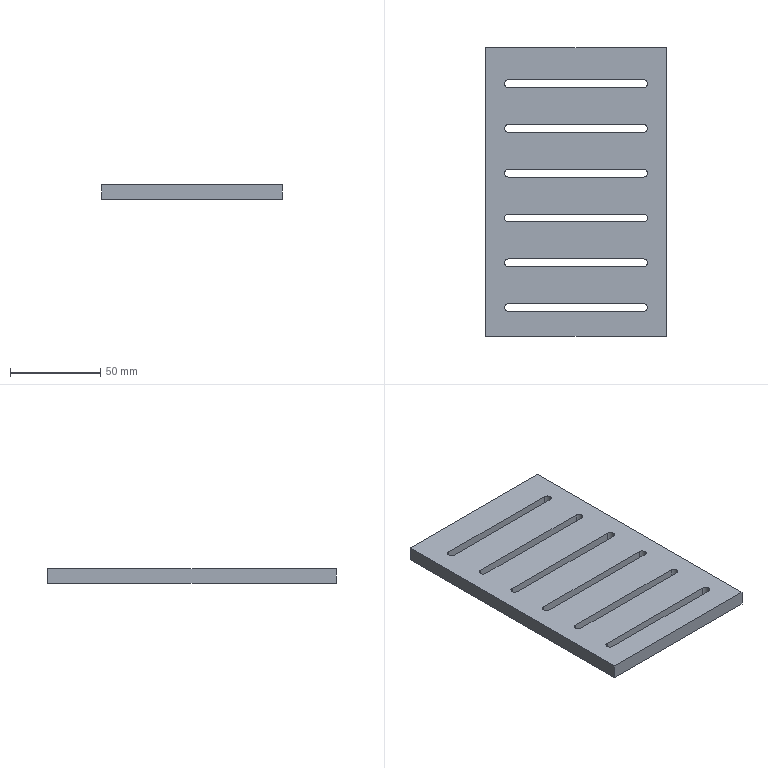Part | STEP file | SynoNew-0304-040 | 1 solid | 38 faces | box 100 x 160 x 8 mm | volume 111423 mm3 | plane 18 | cylinder 16 | cone 4 | commonest cylinder face diameters 4.3 x12 3.242 x4
STEP:
#1=CARTESIAN_POINT('',(-11.379,68.2,4.));
#2=VERTEX_POINT('',#1);
#3=CARTESIAN_POINT('',(-14.621,68.2,4.));
#4=VERTEX_POINT('',#3);
#5=CARTESIAN_POINT('',(-13.,68.2,4.));
#6=DIRECTION('',(0.,1.,0.));
#7=DIRECTION('',(1.,0.,0.));
#8=AXIS2_PLACEMENT_3D('',#5,#6,#7);
#9=CIRCLE('',#8,1.621);
#10=EDGE_CURVE('',#2,#4,#9,.T.);
#11=ORIENTED_EDGE('',*,*,#10,.T.);
#12=CARTESIAN_POINT('',(-13.,67.226,4.));
#13=VERTEX_POINT('',#12);
#14=CARTESIAN_POINT('',(-13.81,67.713,4.));
#15=DIRECTION('',(0.8572,-0.515,0.));
#16=VECTOR('',#15,0.8105);
#17=LINE('',#14,#16);
#18=EDGE_CURVE('',#4,#13,#17,.T.);
#19=ORIENTED_EDGE('',*,*,#18,.T.);
#20=ORIENTED_EDGE('',*,*,#18,.F.);
#21=CARTESIAN_POINT('',(-13.,68.2,4.));
#22=DIRECTION('',(0.,1.,0.));
#23=DIRECTION('',(1.,0.,0.));
#24=AXIS2_PLACEMENT_3D('',#21,#22,#23);
#25=CIRCLE('',#24,1.621);
#26=EDGE_CURVE('',#4,#2,#25,.T.);
#27=ORIENTED_EDGE('',*,*,#26,.T.);
#28=EDGE_LOOP('',(#11,#19,#20,#27));
#29=FACE_OUTER_BOUND('',#28,.T.);
#30=CARTESIAN_POINT('',(-13.,67.713,4.));
#31=DIRECTION('',(0.,1.,0.));
#32=DIRECTION('',(1.,0.,0.));
#33=AXIS2_PLACEMENT_3D('',#30,#31,#32);
#34=CONICAL_SURFACE('',#33,0.8105,1.03);
#35=ADVANCED_FACE('',(#29),#34,.F.);
#36=CARTESIAN_POINT('',(-11.379,80.,4.));
#37=VERTEX_POINT('',#36);
#38=CARTESIAN_POINT('',(-14.621,80.,4.));
#39=VERTEX_POINT('',#38);
#40=CARTESIAN_POINT('',(-13.,80.,4.));
#41=DIRECTION('',(0.,-1.,0.));
#42=DIRECTION('',(1.,0.,0.));
#43=AXIS2_PLACEMENT_3D('',#40,#41,#42);
#44=CIRCLE('',#43,1.621);
#45=EDGE_CURVE('',#37,#39,#44,.T.);
#46=ORIENTED_EDGE('',*,*,#45,.F.);
#47=CARTESIAN_POINT('',(-13.,80.,4.));
#48=DIRECTION('',(0.,-1.,0.));
#49=DIRECTION('',(1.,0.,0.));
#50=AXIS2_PLACEMENT_3D('',#47,#48,#49);
#51=CIRCLE('',#50,1.621);
#52=EDGE_CURVE('',#39,#37,#51,.T.);
#53=ORIENTED_EDGE('',*,*,#52,.F.);
#54=CARTESIAN_POINT('',(-14.621,74.1,4.));
#55=DIRECTION('',(0.,-1.,0.));
#56=VECTOR('',#55,1.621);
#57=LINE('',#54,#56);
#58=EDGE_CURVE('',#39,#4,#57,.T.);
#59=ORIENTED_EDGE('',*,*,#58,.T.);
#60=ORIENTED_EDGE('',*,*,#10,.F.);
#61=ORIENTED_EDGE('',*,*,#26,.F.);
#62=ORIENTED_EDGE('',*,*,#58,.F.);
#63=EDGE_LOOP('',(#46,#53,#59,#60,#61,#62));
#64=FACE_OUTER_BOUND('',#63,.T.);
#65=CARTESIAN_POINT('',(-13.,74.1,4.));
#66=DIRECTION('',(0.,1.,0.));
#67=DIRECTION('',(1.,0.,0.));
#68=AXIS2_PLACEMENT_3D('',#65,#66,#67);
#69=CYLINDRICAL_SURFACE('',#68,1.621);
#70=ADVANCED_FACE('',(#64),#69,.F.);
#71=CARTESIAN_POINT('',(39.621,68.2,4.));
#72=VERTEX_POINT('',#71);
#73=CARTESIAN_POINT('',(36.379,68.2,4.));
#74=VERTEX_POINT('',#73);
#75=CARTESIAN_POINT('',(38.,68.2,4.));
#76=DIRECTION('',(0.,1.,0.));
#77=DIRECTION('',(1.,0.,0.));
#78=AXIS2_PLACEMENT_3D('',#75,#76,#77);
#79=CIRCLE('',#78,1.621);
#80=EDGE_CURVE('',#72,#74,#79,.T.);
#81=ORIENTED_EDGE('',*,*,#80,.T.);
#82=CARTESIAN_POINT('',(38.,67.226,4.));
#83=VERTEX_POINT('',#82);
#84=CARTESIAN_POINT('',(37.19,67.713,4.));
#85=DIRECTION('',(0.8572,-0.515,0.));
#86=VECTOR('',#85,0.8105);
#87=LINE('',#84,#86);
#88=EDGE_CURVE('',#74,#83,#87,.T.);
#89=ORIENTED_EDGE('',*,*,#88,.T.);
#90=ORIENTED_EDGE('',*,*,#88,.F.);
#91=CARTESIAN_POINT('',(38.,68.2,4.));
#92=DIRECTION('',(0.,1.,0.));
#93=DIRECTION('',(1.,0.,0.));
#94=AXIS2_PLACEMENT_3D('',#91,#92,#93);
#95=CIRCLE('',#94,1.621);
#96=EDGE_CURVE('',#74,#72,#95,.T.);
#97=ORIENTED_EDGE('',*,*,#96,.T.);
#98=EDGE_LOOP('',(#81,#89,#90,#97));
#99=FACE_OUTER_BOUND('',#98,.T.);
#100=CARTESIAN_POINT('',(38.,67.713,4.));
#101=DIRECTION('',(0.,1.,0.));
#102=DIRECTION('',(1.,0.,0.));
#103=AXIS2_PLACEMENT_3D('',#100,#101,#102);
#104=CONICAL_SURFACE('',#103,0.8105,1.03);
#105=ADVANCED_FACE('',(#99),#104,.F.);
#106=CARTESIAN_POINT('',(39.621,80.,4.));
#107=VERTEX_POINT('',#106);
#108=CARTESIAN_POINT('',(36.379,80.,4.));
#109=VERTEX_POINT('',#108);
#110=CARTESIAN_POINT('',(38.,80.,4.));
#111=DIRECTION('',(0.,-1.,0.));
#112=DIRECTION('',(1.,0.,0.));
#113=AXIS2_PLACEMENT_3D('',#110,#111,#112);
#114=CIRCLE('',#113,1.621);
#115=EDGE_CURVE('',#107,#109,#114,.T.);
#116=ORIENTED_EDGE('',*,*,#115,.F.);
#117=CARTESIAN_POINT('',(38.,80.,4.));
#118=DIRECTION('',(0.,-1.,0.));
#119=DIRECTION('',(1.,0.,0.));
#120=AXIS2_PLACEMENT_3D('',#117,#118,#119);
#121=CIRCLE('',#120,1.621);
#122=EDGE_CURVE('',#109,#107,#121,.T.);
#123=ORIENTED_EDGE('',*,*,#122,.F.);
#124=CARTESIAN_POINT('',(36.379,74.1,4.));
#125=DIRECTION('',(0.,-1.,0.));
#126=VECTOR('',#125,1.621);
#127=LINE('',#124,#126);
#128=EDGE_CURVE('',#109,#74,#127,.T.);
#129=ORIENTED_EDGE('',*,*,#128,.T.);
#130=ORIENTED_EDGE('',*,*,#80,.F.);
#131=ORIENTED_EDGE('',*,*,#96,.F.);
#132=ORIENTED_EDGE('',*,*,#128,.F.);
#133=EDGE_LOOP('',(#116,#123,#129,#130,#131,#132));
#134=FACE_OUTER_BOUND('',#133,.T.);
#135=CARTESIAN_POINT('',(38.,74.1,4.));
#136=DIRECTION('',(0.,1.,0.));
#137=DIRECTION('',(1.,0.,0.));
#138=AXIS2_PLACEMENT_3D('',#135,#136,#137);
#139=CYLINDRICAL_SURFACE('',#138,1.621);
#140=ADVANCED_FACE('',(#134),#139,.F.);
#141=CARTESIAN_POINT('',(14.621,68.2,4.));
#142=VERTEX_POINT('',#141);
#143=CARTESIAN_POINT('',(11.379,68.2,4.));
#144=VERTEX_POINT('',#143);
#145=CARTESIAN_POINT('',(13.,68.2,4.));
#146=DIRECTION('',(0.,1.,0.));
#147=DIRECTION('',(1.,0.,0.));
#148=AXIS2_PLACEMENT_3D('',#145,#146,#147);
#149=CIRCLE('',#148,1.621);
#150=EDGE_CURVE('',#142,#144,#149,.T.);
#151=ORIENTED_EDGE('',*,*,#150,.T.);
#152=CARTESIAN_POINT('',(13.,67.226,4.));
#153=VERTEX_POINT('',#152);
#154=CARTESIAN_POINT('',(12.19,67.713,4.));
#155=DIRECTION('',(0.8572,-0.515,0.));
#156=VECTOR('',#155,0.8105);
#157=LINE('',#154,#156);
#158=EDGE_CURVE('',#144,#153,#157,.T.);
#159=ORIENTED_EDGE('',*,*,#158,.T.);
#160=ORIENTED_EDGE('',*,*,#158,.F.);
#161=CARTESIAN_POINT('',(13.,68.2,4.));
#162=DIRECTION('',(0.,1.,0.));
#163=DIRECTION('',(1.,0.,0.));
#164=AXIS2_PLACEMENT_3D('',#161,#162,#163);
#165=CIRCLE('',#164,1.621);
#166=EDGE_CURVE('',#144,#142,#165,.T.);
#167=ORIENTED_EDGE('',*,*,#166,.T.);
#168=EDGE_LOOP('',(#151,#159,#160,#167));
#169=FACE_OUTER_BOUND('',#168,.T.);
#170=CARTESIAN_POINT('',(13.,67.713,4.));
#171=DIRECTION('',(0.,1.,0.));
#172=DIRECTION('',(1.,0.,0.));
#173=AXIS2_PLACEMENT_3D('',#170,#171,#172);
#174=CONICAL_SURFACE('',#173,0.8105,1.03);
#175=ADVANCED_FACE('',(#169),#174,.F.);
#176=CARTESIAN_POINT('',(14.621,80.,4.));
#177=VERTEX_POINT('',#176);
#178=CARTESIAN_POINT('',(11.379,80.,4.));
#179=VERTEX_POINT('',#178);
#180=CARTESIAN_POINT('',(13.,80.,4.));
#181=DIRECTION('',(0.,-1.,0.));
#182=DIRECTION('',(1.,0.,0.));
#183=AXIS2_PLACEMENT_3D('',#180,#181,#182);
#184=CIRCLE('',#183,1.621);
#185=EDGE_CURVE('',#177,#179,#184,.T.);
#186=ORIENTED_EDGE('',*,*,#185,.F.);
#187=CARTESIAN_POINT('',(13.,80.,4.));
#188=DIRECTION('',(0.,-1.,0.));
#189=DIRECTION('',(1.,0.,0.));
#190=AXIS2_PLACEMENT_3D('',#187,#188,#189);
#191=CIRCLE('',#190,1.621);
#192=EDGE_CURVE('',#179,#177,#191,.T.);
#193=ORIENTED_EDGE('',*,*,#192,.F.);
#194=CARTESIAN_POINT('',(11.379,74.1,4.));
#195=DIRECTION('',(0.,-1.,0.));
#196=VECTOR('',#195,1.621);
#197=LINE('',#194,#196);
#198=EDGE_CURVE('',#179,#144,#197,.T.);
#199=ORIENTED_EDGE('',*,*,#198,.T.);
#200=ORIENTED_EDGE('',*,*,#150,.F.);
#201=ORIENTED_EDGE('',*,*,#166,.F.);
#202=ORIENTED_EDGE('',*,*,#198,.F.);
#203=EDGE_LOOP('',(#186,#193,#199,#200,#201,#202));
#204=FACE_OUTER_BOUND('',#203,.T.);
#205=CARTESIAN_POINT('',(13.,74.1,4.));
#206=DIRECTION('',(0.,1.,0.));
#207=DIRECTION('',(1.,0.,0.));
#208=AXIS2_PLACEMENT_3D('',#205,#206,#207);
#209=CYLINDRICAL_SURFACE('',#208,1.621);
#210=ADVANCED_FACE('',(#204),#209,.F.);
#211=CARTESIAN_POINT('',(-36.379,68.2,4.));
#212=VERTEX_POINT('',#211);
#213=CARTESIAN_POINT('',(-39.621,68.2,4.));
#214=VERTEX_POINT('',#213);
#215=CARTESIAN_POINT('',(-38.,68.2,4.));
#216=DIRECTION('',(0.,1.,0.));
#217=DIRECTION('',(1.,0.,0.));
#218=AXIS2_PLACEMENT_3D('',#215,#216,#217);
#219=CIRCLE('',#218,1.621);
#220=EDGE_CURVE('',#212,#214,#219,.T.);
#221=ORIENTED_EDGE('',*,*,#220,.T.);
#222=CARTESIAN_POINT('',(-38.,67.226,4.));
#223=VERTEX_POINT('',#222);
#224=CARTESIAN_POINT('',(-38.81,67.713,4.));
#225=DIRECTION('',(0.8572,-0.515,0.));
#226=VECTOR('',#225,0.8105);
#227=LINE('',#224,#226);
#228=EDGE_CURVE('',#214,#223,#227,.T.);
#229=ORIENTED_EDGE('',*,*,#228,.T.);
#230=ORIENTED_EDGE('',*,*,#228,.F.);
#231=CARTESIAN_POINT('',(-38.,68.2,4.));
#232=DIRECTION('',(0.,1.,0.));
#233=DIRECTION('',(1.,0.,0.));
#234=AXIS2_PLACEMENT_3D('',#231,#232,#233);
#235=CIRCLE('',#234,1.621);
#236=EDGE_CURVE('',#214,#212,#235,.T.);
#237=ORIENTED_EDGE('',*,*,#236,.T.);
#238=EDGE_LOOP('',(#221,#229,#230,#237));
#239=FACE_OUTER_BOUND('',#238,.T.);
#240=CARTESIAN_POINT('',(-38.,67.713,4.));
#241=DIRECTION('',(0.,1.,0.));
#242=DIRECTION('',(1.,0.,0.));
#243=AXIS2_PLACEMENT_3D('',#240,#241,#242);
#244=CONICAL_SURFACE('',#243,0.8105,1.03);
#245=ADVANCED_FACE('',(#239),#244,.F.);
#246=CARTESIAN_POINT('',(-36.379,80.,4.));
#247=VERTEX_POINT('',#246);
#248=CARTESIAN_POINT('',(-39.621,80.,4.));
#249=VERTEX_POINT('',#248);
#250=CARTESIAN_POINT('',(-38.,80.,4.));
#251=DIRECTION('',(0.,-1.,0.));
#252=DIRECTION('',(1.,0.,0.));
#253=AXIS2_PLACEMENT_3D('',#250,#251,#252);
#254=CIRCLE('',#253,1.621);
#255=EDGE_CURVE('',#247,#249,#254,.T.);
#256=ORIENTED_EDGE('',*,*,#255,.F.);
#257=CARTESIAN_POINT('',(-38.,80.,4.));
#258=DIRECTION('',(0.,-1.,0.));
#259=DIRECTION('',(1.,0.,0.));
#260=AXIS2_PLACEMENT_3D('',#257,#258,#259);
#261=CIRCLE('',#260,1.621);
#262=EDGE_CURVE('',#249,#247,#261,.T.);
#263=ORIENTED_EDGE('',*,*,#262,.F.);
#264=CARTESIAN_POINT('',(-39.621,74.1,4.));
#265=DIRECTION('',(0.,-1.,0.));
#266=VECTOR('',#265,1.621);
#267=LINE('',#264,#266);
#268=EDGE_CURVE('',#249,#214,#267,.T.);
#269=ORIENTED_EDGE('',*,*,#268,.T.);
#270=ORIENTED_EDGE('',*,*,#220,.F.);
#271=ORIENTED_EDGE('',*,*,#236,.F.);
#272=ORIENTED_EDGE('',*,*,#268,.F.);
#273=EDGE_LOOP('',(#256,#263,#269,#270,#271,#272));
#274=FACE_OUTER_BOUND('',#273,.T.);
#275=CARTESIAN_POINT('',(-38.,74.1,4.));
#276=DIRECTION('',(0.,1.,0.));
#277=DIRECTION('',(1.,0.,0.));
#278=AXIS2_PLACEMENT_3D('',#275,#276,#277);
#279=CYLINDRICAL_SURFACE('',#278,1.621);
#280=ADVANCED_FACE('',(#274),#279,.F.);
#281=CARTESIAN_POINT('',(-37.5,57.85,0.));
#282=VERTEX_POINT('',#281);
#283=CARTESIAN_POINT('',(37.5,57.85,0.));
#284=VERTEX_POINT('',#283);
#285=CARTESIAN_POINT('',(18.75,57.85,0.));
#286=DIRECTION('',(1.,0.,0.));
#287=VECTOR('',#286,10.);
#288=LINE('',#285,#287);
#289=EDGE_CURVE('',#282,#284,#288,.T.);
#290=ORIENTED_EDGE('',*,*,#289,.F.);
#291=CARTESIAN_POINT('',(-37.5,57.85,8.));
#292=VERTEX_POINT('',#291);
#293=CARTESIAN_POINT('',(-37.5,57.85,8.));
#294=DIRECTION('',(0.,0.,-1.));
#295=VECTOR('',#294,10.);
#296=LINE('',#293,#295);
#297=EDGE_CURVE('',#292,#282,#296,.T.);
#298=ORIENTED_EDGE('',*,*,#297,.F.);
#299=CARTESIAN_POINT('',(37.5,57.85,8.));
#300=VERTEX_POINT('',#299);
#301=CARTESIAN_POINT('',(18.75,57.85,8.));
#302=DIRECTION('',(-1.,0.,0.));
#303=VECTOR('',#302,10.);
#304=LINE('',#301,#303);
#305=EDGE_CURVE('',#300,#292,#304,.T.);
#306=ORIENTED_EDGE('',*,*,#305,.F.);
#307=CARTESIAN_POINT('',(37.5,57.85,8.));
#308=DIRECTION('',(0.,0.,-1.));
#309=VECTOR('',#308,10.);
#310=LINE('',#307,#309);
#311=EDGE_CURVE('',#300,#284,#310,.T.);
#312=ORIENTED_EDGE('',*,*,#311,.T.);
#313=EDGE_LOOP('',(#290,#298,#306,#312));
#314=FACE_OUTER_BOUND('',#313,.T.);
#315=CARTESIAN_POINT('',(37.5,57.85,8.));
#316=DIRECTION('',(0.,-1.,0.));
#317=DIRECTION('',(-1.,0.,0.));
#318=AXIS2_PLACEMENT_3D('',#315,#316,#317);
#319=PLANE('',#318);
#320=ADVANCED_FACE('',(#314),#319,.F.);
#321=CARTESIAN_POINT('',(37.5,62.15,0.));
#322=VERTEX_POINT('',#321);
#323=CARTESIAN_POINT('',(37.5,60.,0.));
#324=DIRECTION('',(0.,0.,1.));
#325=DIRECTION('',(0.,-1.,0.));
#326=AXIS2_PLACEMENT_3D('',#323,#324,#325);
#327=CIRCLE('',#326,2.15);
#328=EDGE_CURVE('',#284,#322,#327,.T.);
#329=ORIENTED_EDGE('',*,*,#328,.F.);
#330=ORIENTED_EDGE('',*,*,#311,.F.);
#331=CARTESIAN_POINT('',(37.5,62.15,8.));
#332=VERTEX_POINT('',#331);
#333=CARTESIAN_POINT('',(37.5,60.,8.));
#334=DIRECTION('',(0.,0.,-1.));
#335=DIRECTION('',(0.,-1.,0.));
#336=AXIS2_PLACEMENT_3D('',#333,#334,#335);
#337=CIRCLE('',#336,2.15);
#338=EDGE_CURVE('',#332,#300,#337,.T.);
#339=ORIENTED_EDGE('',*,*,#338,.F.);
#340=CARTESIAN_POINT('',(37.5,62.15,8.));
#341=DIRECTION('',(0.,0.,-1.));
#342=VECTOR('',#341,10.);
#343=LINE('',#340,#342);
#344=EDGE_CURVE('',#332,#322,#343,.T.);
#345=ORIENTED_EDGE('',*,*,#344,.T.);
#346=EDGE_LOOP('',(#329,#330,#339,#345));
#347=FACE_OUTER_BOUND('',#346,.T.);
#348=CARTESIAN_POINT('',(37.5,60.,8.));
#349=DIRECTION('',(0.,0.,-1.));
#350=DIRECTION('',(0.,-1.,0.));
#351=AXIS2_PLACEMENT_3D('',#348,#349,#350);
#352=CYLINDRICAL_SURFACE('',#351,2.15);
#353=ADVANCED_FACE('',(#347),#352,.F.);
#354=CARTESIAN_POINT('',(-37.5,62.15,0.));
#355=VERTEX_POINT('',#354);
#356=CARTESIAN_POINT('',(-18.75,62.15,0.));
#357=DIRECTION('',(-1.,0.,0.));
#358=VECTOR('',#357,10.);
#359=LINE('',#356,#358);
#360=EDGE_CURVE('',#322,#355,#359,.T.);
#361=ORIENTED_EDGE('',*,*,#360,.F.);
#362=ORIENTED_EDGE('',*,*,#344,.F.);
#363=CARTESIAN_POINT('',(-37.5,62.15,8.));
#364=VERTEX_POINT('',#363);
#365=CARTESIAN_POINT('',(-18.75,62.15,8.));
#366=DIRECTION('',(1.,0.,0.));
#367=VECTOR('',#366,10.);
#368=LINE('',#365,#367);
#369=EDGE_CURVE('',#364,#332,#368,.T.);
#370=ORIENTED_EDGE('',*,*,#369,.F.);
#371=CARTESIAN_POINT('',(-37.5,62.15,8.));
#372=DIRECTION('',(0.,0.,-1.));
#373=VECTOR('',#372,10.);
#374=LINE('',#371,#373);
#375=EDGE_CURVE('',#364,#355,#374,.T.);
#376=ORIENTED_EDGE('',*,*,#375,.T.);
#377=EDGE_LOOP('',(#361,#362,#370,#376));
#378=FACE_OUTER_BOUND('',#377,.T.);
#379=CARTESIAN_POINT('',(-37.5,62.15,8.));
#380=DIRECTION('',(0.,1.,0.));
#381=DIRECTION('',(1.,0.,0.));
#382=AXIS2_PLACEMENT_3D('',#379,#380,#381);
#383=PLANE('',#382);
#384=ADVANCED_FACE('',(#378),#383,.F.);
#385=CARTESIAN_POINT('',(-37.5,60.,0.));
#386=DIRECTION('',(0.,0.,1.));
#387=DIRECTION('',(0.,1.,0.));
#388=AXIS2_PLACEMENT_3D('',#385,#386,#387);
#389=CIRCLE('',#388,2.15);
#390=EDGE_CURVE('',#355,#282,#389,.T.);
#391=ORIENTED_EDGE('',*,*,#390,.F.);
#392=ORIENTED_EDGE('',*,*,#375,.F.);
#393=CARTESIAN_POINT('',(-37.5,60.,8.));
#394=DIRECTION('',(0.,0.,-1.));
#395=DIRECTION('',(0.,1.,0.));
#396=AXIS2_PLACEMENT_3D('',#393,#394,#395);
#397=CIRCLE('',#396,2.15);
#398=EDGE_CURVE('',#292,#364,#397,.T.);
#399=ORIENTED_EDGE('',*,*,#398,.F.);
#400=ORIENTED_EDGE('',*,*,#297,.T.);
#401=EDGE_LOOP('',(#391,#392,#399,#400));
#402=FACE_OUTER_BOUND('',#401,.T.);
#403=CARTESIAN_POINT('',(-37.5,60.,8.));
#404=DIRECTION('',(0.,0.,-1.));
#405=DIRECTION('',(0.,1.,0.));
#406=AXIS2_PLACEMENT_3D('',#403,#404,#405);
#407=CYLINDRICAL_SURFACE('',#406,2.15);
#408=ADVANCED_FACE('',(#402),#407,.F.);
#409=CARTESIAN_POINT('',(-37.5,33.05,0.));
#410=VERTEX_POINT('',#409);
#411=CARTESIAN_POINT('',(37.5,33.05,0.));
#412=VERTEX_POINT('',#411);
#413=CARTESIAN_POINT('',(18.75,33.05,0.));
#414=DIRECTION('',(1.,0.,0.));
#415=VECTOR('',#414,10.);
#416=LINE('',#413,#415);
#417=EDGE_CURVE('',#410,#412,#416,.T.);
#418=ORIENTED_EDGE('',*,*,#417,.F.);
#419=CARTESIAN_POINT('',(-37.5,33.05,8.));
#420=VERTEX_POINT('',#419);
#421=CARTESIAN_POINT('',(-37.5,33.05,8.));
#422=DIRECTION('',(0.,0.,-1.));
#423=VECTOR('',#422,10.);
#424=LINE('',#421,#423);
#425=EDGE_CURVE('',#420,#410,#424,.T.);
#426=ORIENTED_EDGE('',*,*,#425,.F.);
#427=CARTESIAN_POINT('',(37.5,33.05,8.));
#428=VERTEX_POINT('',#427);
#429=CARTESIAN_POINT('',(18.75,33.05,8.));
#430=DIRECTION('',(-1.,0.,0.));
#431=VECTOR('',#430,10.);
#432=LINE('',#429,#431);
#433=EDGE_CURVE('',#428,#420,#432,.T.);
#434=ORIENTED_EDGE('',*,*,#433,.F.);
#435=CARTESIAN_POINT('',(37.5,33.05,8.));
#436=DIRECTION('',(0.,0.,-1.));
#437=VECTOR('',#436,10.);
#438=LINE('',#435,#437);
#439=EDGE_CURVE('',#428,#412,#438,.T.);
#440=ORIENTED_EDGE('',*,*,#439,.T.);
#441=EDGE_LOOP('',(#418,#426,#434,#440));
#442=FACE_OUTER_BOUND('',#441,.T.);
#443=CARTESIAN_POINT('',(37.5,33.05,8.));
#444=DIRECTION('',(0.,-1.,0.));
#445=DIRECTION('',(-1.,0.,0.));
#446=AXIS2_PLACEMENT_3D('',#443,#444,#445);
#447=PLANE('',#446);
#448=ADVANCED_FACE('',(#442),#447,.F.);
#449=CARTESIAN_POINT('',(37.5,37.35,0.));
#450=VERTEX_POINT('',#449);
#451=CARTESIAN_POINT('',(37.5,35.2,0.));
#452=DIRECTION('',(0.,0.,1.));
#453=DIRECTION('',(0.,-1.,0.));
#454=AXIS2_PLACEMENT_3D('',#451,#452,#453);
#455=CIRCLE('',#454,2.15);
#456=EDGE_CURVE('',#412,#450,#455,.T.);
#457=ORIENTED_EDGE('',*,*,#456,.F.);
#458=ORIENTED_EDGE('',*,*,#439,.F.);
#459=CARTESIAN_POINT('',(37.5,37.35,8.));
#460=VERTEX_POINT('',#459);
#461=CARTESIAN_POINT('',(37.5,35.2,8.));
#462=DIRECTION('',(0.,0.,-1.));
#463=DIRECTION('',(0.,-1.,0.));
#464=AXIS2_PLACEMENT_3D('',#461,#462,#463);
#465=CIRCLE('',#464,2.15);
#466=EDGE_CURVE('',#460,#428,#465,.T.);
#467=ORIENTED_EDGE('',*,*,#466,.F.);
#468=CARTESIAN_POINT('',(37.5,37.35,8.));
#469=DIRECTION('',(0.,0.,-1.));
#470=VECTOR('',#469,10.);
#471=LINE('',#468,#470);
#472=EDGE_CURVE('',#460,#450,#471,.T.);
#473=ORIENTED_EDGE('',*,*,#472,.T.);
#474=EDGE_LOOP('',(#457,#458,#467,#473));
#475=FACE_OUTER_BOUND('',#474,.T.);
#476=CARTESIAN_POINT('',(37.5,35.2,8.));
#477=DIRECTION('',(0.,0.,-1.));
#478=DIRECTION('',(0.,-1.,0.));
#479=AXIS2_PLACEMENT_3D('',#476,#477,#478);
#480=CYLINDRICAL_SURFACE('',#479,2.15);
#481=ADVANCED_FACE('',(#475),#480,.F.);
#482=CARTESIAN_POINT('',(-37.5,37.35,0.));
#483=VERTEX_POINT('',#482);
#484=CARTESIAN_POINT('',(-18.75,37.35,0.));
#485=DIRECTION('',(-1.,0.,0.));
#486=VECTOR('',#485,10.);
#487=LINE('',#484,#486);
#488=EDGE_CURVE('',#450,#483,#487,.T.);
#489=ORIENTED_EDGE('',*,*,#488,.F.);
#490=ORIENTED_EDGE('',*,*,#472,.F.);
#491=CARTESIAN_POINT('',(-37.5,37.35,8.));
#492=VERTEX_POINT('',#491);
#493=CARTESIAN_POINT('',(-18.75,37.35,8.));
#494=DIRECTION('',(1.,0.,0.));
#495=VECTOR('',#494,10.);
#496=LINE('',#493,#495);
#497=EDGE_CURVE('',#492,#460,#496,.T.);
#498=ORIENTED_EDGE('',*,*,#497,.F.);
#499=CARTESIAN_POINT('',(-37.5,37.35,8.));
#500=DIRECTION('',(0.,0.,-1.));
#501=VECTOR('',#500,10.);
#502=LINE('',#499,#501);
#503=EDGE_CURVE('',#492,#483,#502,.T.);
#504=ORIENTED_EDGE('',*,*,#503,.T.);
#505=EDGE_LOOP('',(#489,#490,#498,#504));
#506=FACE_OUTER_BOUND('',#505,.T.);
#507=CARTESIAN_POINT('',(-37.5,37.35,8.));
#508=DIRECTION('',(0.,1.,0.));
#509=DIRECTION('',(1.,0.,0.));
#510=AXIS2_PLACEMENT_3D('',#507,#508,#509);
#511=PLANE('',#510);
#512=ADVANCED_FACE('',(#506),#511,.F.);
#513=CARTESIAN_POINT('',(-37.5,35.2,0.));
#514=DIRECTION('',(0.,0.,1.));
#515=DIRECTION('',(0.,1.,0.));
#516=AXIS2_PLACEMENT_3D('',#513,#514,#515);
#517=CIRCLE('',#516,2.15);
#518=EDGE_CURVE('',#483,#410,#517,.T.);
#519=ORIENTED_EDGE('',*,*,#518,.F.);
#520=ORIENTED_EDGE('',*,*,#503,.F.);
#521=CARTESIAN_POINT('',(-37.5,35.2,8.));
#522=DIRECTION('',(0.,0.,-1.));
#523=DIRECTION('',(0.,1.,0.));
#524=AXIS2_PLACEMENT_3D('',#521,#522,#523);
#525=CIRCLE('',#524,2.15);
#526=EDGE_CURVE('',#420,#492,#525,.T.);
#527=ORIENTED_EDGE('',*,*,#526,.F.);
#528=ORIENTED_EDGE('',*,*,#425,.T.);
#529=EDGE_LOOP('',(#519,#520,#527,#528));
#530=FACE_OUTER_BOUND('',#529,.T.);
#531=CARTESIAN_POINT('',(-37.5,35.2,8.));
#532=DIRECTION('',(0.,0.,-1.));
#533=DIRECTION('',(0.,1.,0.));
#534=AXIS2_PLACEMENT_3D('',#531,#532,#533);
#535=CYLINDRICAL_SURFACE('',#534,2.15);
#536=ADVANCED_FACE('',(#530),#535,.F.);
#537=CARTESIAN_POINT('',(-37.5,8.25,0.));
#538=VERTEX_POINT('',#537);
#539=CARTESIAN_POINT('',(37.5,8.25,0.));
#540=VERTEX_POINT('',#539);
#541=CARTESIAN_POINT('',(18.75,8.25,0.));
#542=DIRECTION('',(1.,0.,0.));
#543=VECTOR('',#542,10.);
#544=LINE('',#541,#543);
#545=EDGE_CURVE('',#538,#540,#544,.T.);
#546=ORIENTED_EDGE('',*,*,#545,.F.);
#547=CARTESIAN_POINT('',(-37.5,8.25,8.));
#548=VERTEX_POINT('',#547);
#549=CARTESIAN_POINT('',(-37.5,8.25,8.));
#550=DIRECTION('',(0.,0.,-1.));
#551=VECTOR('',#550,10.);
#552=LINE('',#549,#551);
#553=EDGE_CURVE('',#548,#538,#552,.T.);
#554=ORIENTED_EDGE('',*,*,#553,.F.);
#555=CARTESIAN_POINT('',(37.5,8.25,8.));
#556=VERTEX_POINT('',#555);
#557=CARTESIAN_POINT('',(18.75,8.25,8.));
#558=DIRECTION('',(-1.,0.,0.));
#559=VECTOR('',#558,10.);
#560=LINE('',#557,#559);
#561=EDGE_CURVE('',#556,#548,#560,.T.);
#562=ORIENTED_EDGE('',*,*,#561,.F.);
#563=CARTESIAN_POINT('',(37.5,8.25,8.));
#564=DIRECTION('',(0.,0.,-1.));
#565=VECTOR('',#564,10.);
#566=LINE('',#563,#565);
#567=EDGE_CURVE('',#556,#540,#566,.T.);
#568=ORIENTED_EDGE('',*,*,#567,.T.);
#569=EDGE_LOOP('',(#546,#554,#562,#568));
#570=FACE_OUTER_BOUND('',#569,.T.);
#571=CARTESIAN_POINT('',(37.5,8.25,8.));
#572=DIRECTION('',(0.,-1.,0.));
#573=DIRECTION('',(-1.,0.,0.));
#574=AXIS2_PLACEMENT_3D('',#571,#572,#573);
#575=PLANE('',#574);
#576=ADVANCED_FACE('',(#570),#575,.F.);
#577=CARTESIAN_POINT('',(37.5,12.55,0.));
#578=VERTEX_POINT('',#577);
#579=CARTESIAN_POINT('',(37.5,10.4,0.));
#580=DIRECTION('',(0.,0.,1.));
#581=DIRECTION('',(0.,-1.,0.));
#582=AXIS2_PLACEMENT_3D('',#579,#580,#581);
#583=CIRCLE('',#582,2.15);
#584=EDGE_CURVE('',#540,#578,#583,.T.);
#585=ORIENTED_EDGE('',*,*,#584,.F.);
#586=ORIENTED_EDGE('',*,*,#567,.F.);
#587=CARTESIAN_POINT('',(37.5,12.55,8.));
#588=VERTEX_POINT('',#587);
#589=CARTESIAN_POINT('',(37.5,10.4,8.));
#590=DIRECTION('',(0.,0.,-1.));
#591=DIRECTION('',(0.,-1.,0.));
#592=AXIS2_PLACEMENT_3D('',#589,#590,#591);
#593=CIRCLE('',#592,2.15);
#594=EDGE_CURVE('',#588,#556,#593,.T.);
#595=ORIENTED_EDGE('',*,*,#594,.F.);
#596=CARTESIAN_POINT('',(37.5,12.55,8.));
#597=DIRECTION('',(0.,0.,-1.));
#598=VECTOR('',#597,10.);
#599=LINE('',#596,#598);
#600=EDGE_CURVE('',#588,#578,#599,.T.);
#601=ORIENTED_EDGE('',*,*,#600,.T.);
#602=EDGE_LOOP('',(#585,#586,#595,#601));
#603=FACE_OUTER_BOUND('',#602,.T.);
#604=CARTESIAN_POINT('',(37.5,10.4,8.));
#605=DIRECTION('',(0.,0.,-1.));
#606=DIRECTION('',(0.,-1.,0.));
#607=AXIS2_PLACEMENT_3D('',#604,#605,#606);
#608=CYLINDRICAL_SURFACE('',#607,2.15);
#609=ADVANCED_FACE('',(#603),#608,.F.);
#610=CARTESIAN_POINT('',(-37.5,12.55,0.));
#611=VERTEX_POINT('',#610);
#612=CARTESIAN_POINT('',(-18.75,12.55,0.));
#613=DIRECTION('',(-1.,0.,0.));
#614=VECTOR('',#613,10.);
#615=LINE('',#612,#614);
#616=EDGE_CURVE('',#578,#611,#615,.T.);
#617=ORIENTED_EDGE('',*,*,#616,.F.);
#618=ORIENTED_EDGE('',*,*,#600,.F.);
#619=CARTESIAN_POINT('',(-37.5,12.55,8.));
#620=VERTEX_POINT('',#619);
#621=CARTESIAN_POINT('',(-18.75,12.55,8.));
#622=DIRECTION('',(1.,0.,0.));
#623=VECTOR('',#622,10.);
#624=LINE('',#621,#623);
#625=EDGE_CURVE('',#620,#588,#624,.T.);
#626=ORIENTED_EDGE('',*,*,#625,.F.);
#627=CARTESIAN_POINT('',(-37.5,12.55,8.));
#628=DIRECTION('',(0.,0.,-1.));
#629=VECTOR('',#628,10.);
#630=LINE('',#627,#629);
#631=EDGE_CURVE('',#620,#611,#630,.T.);
#632=ORIENTED_EDGE('',*,*,#631,.T.);
#633=EDGE_LOOP('',(#617,#618,#626,#632));
#634=FACE_OUTER_BOUND('',#633,.T.);
#635=CARTESIAN_POINT('',(-37.5,12.55,8.));
#636=DIRECTION('',(0.,1.,0.));
#637=DIRECTION('',(1.,0.,0.));
#638=AXIS2_PLACEMENT_3D('',#635,#636,#637);
#639=PLANE('',#638);
#640=ADVANCED_FACE('',(#634),#639,.F.);
#641=CARTESIAN_POINT('',(-37.5,10.4,0.));
#642=DIRECTION('',(0.,0.,1.));
#643=DIRECTION('',(0.,1.,0.));
#644=AXIS2_PLACEMENT_3D('',#641,#642,#643);
#645=CIRCLE('',#644,2.15);
#646=EDGE_CURVE('',#611,#538,#645,.T.);
#647=ORIENTED_EDGE('',*,*,#646,.F.);
#648=ORIENTED_EDGE('',*,*,#631,.F.);
#649=CARTESIAN_POINT('',(-37.5,10.4,8.));
#650=DIRECTION('',(0.,0.,-1.));
#651=DIRECTION('',(0.,1.,0.));
#652=AXIS2_PLACEMENT_3D('',#649,#650,#651);
#653=CIRCLE('',#652,2.15);
#654=EDGE_CURVE('',#548,#620,#653,.T.);
#655=ORIENTED_EDGE('',*,*,#654,.F.);
#656=ORIENTED_EDGE('',*,*,#553,.T.);
#657=EDGE_LOOP('',(#647,#648,#655,#656));
#658=FACE_OUTER_BOUND('',#657,.T.);
#659=CARTESIAN_POINT('',(-37.5,10.4,8.));
#660=DIRECTION('',(0.,0.,-1.));
#661=DIRECTION('',(0.,1.,0.));
#662=AXIS2_PLACEMENT_3D('',#659,#660,#661);
#663=CYLINDRICAL_SURFACE('',#662,2.15);
#664=ADVANCED_FACE('',(#658),#663,.F.);
#665=CARTESIAN_POINT('',(-37.5,-16.55,0.));
#666=VERTEX_POINT('',#665);
#667=CARTESIAN_POINT('',(37.5,-16.55,0.));
#668=VERTEX_POINT('',#667);
#669=CARTESIAN_POINT('',(18.75,-16.55,0.));
#670=DIRECTION('',(1.,0.,0.));
#671=VECTOR('',#670,10.);
#672=LINE('',#669,#671);
#673=EDGE_CURVE('',#666,#668,#672,.T.);
#674=ORIENTED_EDGE('',*,*,#673,.F.);
#675=CARTESIAN_POINT('',(-37.5,-16.55,8.));
#676=VERTEX_POINT('',#675);
#677=CARTESIAN_POINT('',(-37.5,-16.55,8.));
#678=DIRECTION('',(0.,0.,-1.));
#679=VECTOR('',#678,10.);
#680=LINE('',#677,#679);
#681=EDGE_CURVE('',#676,#666,#680,.T.);
#682=ORIENTED_EDGE('',*,*,#681,.F.);
#683=CARTESIAN_POINT('',(37.5,-16.55,8.));
#684=VERTEX_POINT('',#683);
#685=CARTESIAN_POINT('',(18.75,-16.55,8.));
#686=DIRECTION('',(-1.,0.,0.));
#687=VECTOR('',#686,10.);
#688=LINE('',#685,#687);
#689=EDGE_CURVE('',#684,#676,#688,.T.);
#690=ORIENTED_EDGE('',*,*,#689,.F.);
#691=CARTESIAN_POINT('',(37.5,-16.55,8.));
#692=DIRECTION('',(0.,0.,-1.));
#693=VECTOR('',#692,10.);
#694=LINE('',#691,#693);
#695=EDGE_CURVE('',#684,#668,#694,.T.);
#696=ORIENTED_EDGE('',*,*,#695,.T.);
#697=EDGE_LOOP('',(#674,#682,#690,#696));
#698=FACE_OUTER_BOUND('',#697,.T.);
#699=CARTESIAN_POINT('',(37.5,-16.55,8.));
#700=DIRECTION('',(0.,-1.,0.));
#701=DIRECTION('',(-1.,0.,0.));
#702=AXIS2_PLACEMENT_3D('',#699,#700,#701);
#703=PLANE('',#702);
#704=ADVANCED_FACE('',(#698),#703,.F.);
#705=CARTESIAN_POINT('',(37.5,-12.25,0.));
#706=VERTEX_POINT('',#705);
#707=CARTESIAN_POINT('',(37.5,-14.4,0.));
#708=DIRECTION('',(0.,0.,1.));
#709=DIRECTION('',(0.,-1.,0.));
#710=AXIS2_PLACEMENT_3D('',#707,#708,#709);
#711=CIRCLE('',#710,2.15);
#712=EDGE_CURVE('',#668,#706,#711,.T.);
#713=ORIENTED_EDGE('',*,*,#712,.F.);
#714=ORIENTED_EDGE('',*,*,#695,.F.);
#715=CARTESIAN_POINT('',(37.5,-12.25,8.));
#716=VERTEX_POINT('',#715);
#717=CARTESIAN_POINT('',(37.5,-14.4,8.));
#718=DIRECTION('',(0.,0.,-1.));
#719=DIRECTION('',(0.,-1.,0.));
#720=AXIS2_PLACEMENT_3D('',#717,#718,#719);
#721=CIRCLE('',#720,2.15);
#722=EDGE_CURVE('',#716,#684,#721,.T.);
#723=ORIENTED_EDGE('',*,*,#722,.F.);
#724=CARTESIAN_POINT('',(37.5,-12.25,8.));
#725=DIRECTION('',(0.,0.,-1.));
#726=VECTOR('',#725,10.);
#727=LINE('',#724,#726);
#728=EDGE_CURVE('',#716,#706,#727,.T.);
#729=ORIENTED_EDGE('',*,*,#728,.T.);
#730=EDGE_LOOP('',(#713,#714,#723,#729));
#731=FACE_OUTER_BOUND('',#730,.T.);
#732=CARTESIAN_POINT('',(37.5,-14.4,8.));
#733=DIRECTION('',(0.,0.,-1.));
#734=DIRECTION('',(0.,-1.,0.));
#735=AXIS2_PLACEMENT_3D('',#732,#733,#734);
#736=CYLINDRICAL_SURFACE('',#735,2.15);
#737=ADVANCED_FACE('',(#731),#736,.F.);
#738=CARTESIAN_POINT('',(-37.5,-12.25,0.));
#739=VERTEX_POINT('',#738);
#740=CARTESIAN_POINT('',(-18.75,-12.25,0.));
#741=DIRECTION('',(-1.,0.,0.));
#742=VECTOR('',#741,10.);
#743=LINE('',#740,#742);
#744=EDGE_CURVE('',#706,#739,#743,.T.);
#745=ORIENTED_EDGE('',*,*,#744,.F.);
#746=ORIENTED_EDGE('',*,*,#728,.F.);
#747=CARTESIAN_POINT('',(-37.5,-12.25,8.));
#748=VERTEX_POINT('',#747);
#749=CARTESIAN_POINT('',(-18.75,-12.25,8.));
#750=DIRECTION('',(1.,0.,0.));
#751=VECTOR('',#750,10.);
#752=LINE('',#749,#751);
#753=EDGE_CURVE('',#748,#716,#752,.T.);
#754=ORIENTED_EDGE('',*,*,#753,.F.);
#755=CARTESIAN_POINT('',(-37.5,-12.25,8.));
#756=DIRECTION('',(0.,0.,-1.));
#757=VECTOR('',#756,10.);
#758=LINE('',#755,#757);
#759=EDGE_CURVE('',#748,#739,#758,.T.);
#760=ORIENTED_EDGE('',*,*,#759,.T.);
#761=EDGE_LOOP('',(#745,#746,#754,#760));
#762=FACE_OUTER_BOUND('',#761,.T.);
#763=CARTESIAN_POINT('',(-37.5,-12.25,8.));
#764=DIRECTION('',(0.,1.,0.));
#765=DIRECTION('',(1.,0.,0.));
#766=AXIS2_PLACEMENT_3D('',#763,#764,#765);
#767=PLANE('',#766);
#768=ADVANCED_FACE('',(#762),#767,.F.);
#769=CARTESIAN_POINT('',(-37.5,-14.4,0.));
#770=DIRECTION('',(0.,0.,1.));
#771=DIRECTION('',(0.,1.,0.));
#772=AXIS2_PLACEMENT_3D('',#769,#770,#771);
#773=CIRCLE('',#772,2.15);
#774=EDGE_CURVE('',#739,#666,#773,.T.);
#775=ORIENTED_EDGE('',*,*,#774,.F.);
#776=ORIENTED_EDGE('',*,*,#759,.F.);
#777=CARTESIAN_POINT('',(-37.5,-14.4,8.));
#778=DIRECTION('',(0.,0.,-1.));
#779=DIRECTION('',(0.,1.,0.));
#780=AXIS2_PLACEMENT_3D('',#777,#778,#779);
#781=CIRCLE('',#780,2.15);
#782=EDGE_CURVE('',#676,#748,#781,.T.);
#783=ORIENTED_EDGE('',*,*,#782,.F.);
#784=ORIENTED_EDGE('',*,*,#681,.T.);
#785=EDGE_LOOP('',(#775,#776,#783,#784));
#786=FACE_OUTER_BOUND('',#785,.T.);
#787=CARTESIAN_POINT('',(-37.5,-14.4,8.));
#788=DIRECTION('',(0.,0.,-1.));
#789=DIRECTION('',(0.,1.,0.));
#790=AXIS2_PLACEMENT_3D('',#787,#788,#789);
#791=CYLINDRICAL_SURFACE('',#790,2.15);
#792=ADVANCED_FACE('',(#786),#791,.F.);
#793=CARTESIAN_POINT('',(-37.5,-41.35,0.));
#794=VERTEX_POINT('',#793);
#795=CARTESIAN_POINT('',(37.5,-41.35,0.));
#796=VERTEX_POINT('',#795);
#797=CARTESIAN_POINT('',(18.75,-41.35,0.));
#798=DIRECTION('',(1.,0.,0.));
#799=VECTOR('',#798,10.);
#800=LINE('',#797,#799);
#801=EDGE_CURVE('',#794,#796,#800,.T.);
#802=ORIENTED_EDGE('',*,*,#801,.F.);
#803=CARTESIAN_POINT('',(-37.5,-41.35,8.));
#804=VERTEX_POINT('',#803);
#805=CARTESIAN_POINT('',(-37.5,-41.35,8.));
#806=DIRECTION('',(0.,0.,-1.));
#807=VECTOR('',#806,10.);
#808=LINE('',#805,#807);
#809=EDGE_CURVE('',#804,#794,#808,.T.);
#810=ORIENTED_EDGE('',*,*,#809,.F.);
#811=CARTESIAN_POINT('',(37.5,-41.35,8.));
#812=VERTEX_POINT('',#811);
#813=CARTESIAN_POINT('',(18.75,-41.35,8.));
#814=DIRECTION('',(-1.,0.,0.));
#815=VECTOR('',#814,10.);
#816=LINE('',#813,#815);
#817=EDGE_CURVE('',#812,#804,#816,.T.);
#818=ORIENTED_EDGE('',*,*,#817,.F.);
#819=CARTESIAN_POINT('',(37.5,-41.35,8.));
#820=DIRECTION('',(0.,0.,-1.));
#821=VECTOR('',#820,10.);
#822=LINE('',#819,#821);
#823=EDGE_CURVE('',#812,#796,#822,.T.);
#824=ORIENTED_EDGE('',*,*,#823,.T.);
#825=EDGE_LOOP('',(#802,#810,#818,#824));
#826=FACE_OUTER_BOUND('',#825,.T.);
#827=CARTESIAN_POINT('',(37.5,-41.35,8.));
#828=DIRECTION('',(0.,-1.,0.));
#829=DIRECTION('',(-1.,0.,0.));
#830=AXIS2_PLACEMENT_3D('',#827,#828,#829);
#831=PLANE('',#830);
#832=ADVANCED_FACE('',(#826),#831,.F.);
#833=CARTESIAN_POINT('',(37.5,-37.05,0.));
#834=VERTEX_POINT('',#833);
#835=CARTESIAN_POINT('',(37.5,-39.2,0.));
#836=DIRECTION('',(0.,0.,1.));
#837=DIRECTION('',(0.,-1.,0.));
#838=AXIS2_PLACEMENT_3D('',#835,#836,#837);
#839=CIRCLE('',#838,2.15);
#840=EDGE_CURVE('',#796,#834,#839,.T.);
#841=ORIENTED_EDGE('',*,*,#840,.F.);
#842=ORIENTED_EDGE('',*,*,#823,.F.);
#843=CARTESIAN_POINT('',(37.5,-37.05,8.));
#844=VERTEX_POINT('',#843);
#845=CARTESIAN_POINT('',(37.5,-39.2,8.));
#846=DIRECTION('',(0.,0.,-1.));
#847=DIRECTION('',(0.,-1.,0.));
#848=AXIS2_PLACEMENT_3D('',#845,#846,#847);
#849=CIRCLE('',#848,2.15);
#850=EDGE_CURVE('',#844,#812,#849,.T.);
#851=ORIENTED_EDGE('',*,*,#850,.F.);
#852=CARTESIAN_POINT('',(37.5,-37.05,8.));
#853=DIRECTION('',(0.,0.,-1.));
#854=VECTOR('',#853,10.);
#855=LINE('',#852,#854);
#856=EDGE_CURVE('',#844,#834,#855,.T.);
#857=ORIENTED_EDGE('',*,*,#856,.T.);
#858=EDGE_LOOP('',(#841,#842,#851,#857));
#859=FACE_OUTER_BOUND('',#858,.T.);
#860=CARTESIAN_POINT('',(37.5,-39.2,8.));
#861=DIRECTION('',(0.,0.,-1.));
#862=DIRECTION('',(0.,-1.,0.));
#863=AXIS2_PLACEMENT_3D('',#860,#861,#862);
#864=CYLINDRICAL_SURFACE('',#863,2.15);
#865=ADVANCED_FACE('',(#859),#864,.F.);
#866=CARTESIAN_POINT('',(-37.5,-37.05,0.));
#867=VERTEX_POINT('',#866);
#868=CARTESIAN_POINT('',(-18.75,-37.05,0.));
#869=DIRECTION('',(-1.,0.,0.));
#870=VECTOR('',#869,10.);
#871=LINE('',#868,#870);
#872=EDGE_CURVE('',#834,#867,#871,.T.);
#873=ORIENTED_EDGE('',*,*,#872,.F.);
#874=ORIENTED_EDGE('',*,*,#856,.F.);
#875=CARTESIAN_POINT('',(-37.5,-37.05,8.));
#876=VERTEX_POINT('',#875);
#877=CARTESIAN_POINT('',(-18.75,-37.05,8.));
#878=DIRECTION('',(1.,0.,0.));
#879=VECTOR('',#878,10.);
#880=LINE('',#877,#879);
#881=EDGE_CURVE('',#876,#844,#880,.T.);
#882=ORIENTED_EDGE('',*,*,#881,.F.);
#883=CARTESIAN_POINT('',(-37.5,-37.05,8.));
#884=DIRECTION('',(0.,0.,-1.));
#885=VECTOR('',#884,10.);
#886=LINE('',#883,#885);
#887=EDGE_CURVE('',#876,#867,#886,.T.);
#888=ORIENTED_EDGE('',*,*,#887,.T.);
#889=EDGE_LOOP('',(#873,#874,#882,#888));
#890=FACE_OUTER_BOUND('',#889,.T.);
#891=CARTESIAN_POINT('',(-37.5,-37.05,8.));
#892=DIRECTION('',(0.,1.,0.));
#893=DIRECTION('',(1.,0.,0.));
#894=AXIS2_PLACEMENT_3D('',#891,#892,#893);
#895=PLANE('',#894);
#896=ADVANCED_FACE('',(#890),#895,.F.);
#897=CARTESIAN_POINT('',(-37.5,-39.2,0.));
#898=DIRECTION('',(0.,0.,1.));
#899=DIRECTION('',(0.,1.,0.));
#900=AXIS2_PLACEMENT_3D('',#897,#898,#899);
#901=CIRCLE('',#900,2.15);
#902=EDGE_CURVE('',#867,#794,#901,.T.);
#903=ORIENTED_EDGE('',*,*,#902,.F.);
#904=ORIENTED_EDGE('',*,*,#887,.F.);
#905=CARTESIAN_POINT('',(-37.5,-39.2,8.));
#906=DIRECTION('',(0.,0.,-1.));
#907=DIRECTION('',(0.,1.,0.));
#908=AXIS2_PLACEMENT_3D('',#905,#906,#907);
#909=CIRCLE('',#908,2.15);
#910=EDGE_CURVE('',#804,#876,#909,.T.);
#911=ORIENTED_EDGE('',*,*,#910,.F.);
#912=ORIENTED_EDGE('',*,*,#809,.T.);
#913=EDGE_LOOP('',(#903,#904,#911,#912));
#914=FACE_OUTER_BOUND('',#913,.T.);
#915=CARTESIAN_POINT('',(-37.5,-39.2,8.));
#916=DIRECTION('',(0.,0.,-1.));
#917=DIRECTION('',(0.,1.,0.));
#918=AXIS2_PLACEMENT_3D('',#915,#916,#917);
#919=CYLINDRICAL_SURFACE('',#918,2.15);
#920=ADVANCED_FACE('',(#914),#919,.F.);
#921=CARTESIAN_POINT('',(-37.5,-66.15,0.));
#922=VERTEX_POINT('',#921);
#923=CARTESIAN_POINT('',(37.5,-66.15,0.));
#924=VERTEX_POINT('',#923);
#925=CARTESIAN_POINT('',(18.75,-66.15,0.));
#926=DIRECTION('',(1.,0.,0.));
#927=VECTOR('',#926,10.);
#928=LINE('',#925,#927);
#929=EDGE_CURVE('',#922,#924,#928,.T.);
#930=ORIENTED_EDGE('',*,*,#929,.F.);
#931=CARTESIAN_POINT('',(-37.5,-66.15,8.));
#932=VERTEX_POINT('',#931);
#933=CARTESIAN_POINT('',(-37.5,-66.15,8.));
#934=DIRECTION('',(0.,0.,-1.));
#935=VECTOR('',#934,10.);
#936=LINE('',#933,#935);
#937=EDGE_CURVE('',#932,#922,#936,.T.);
#938=ORIENTED_EDGE('',*,*,#937,.F.);
#939=CARTESIAN_POINT('',(37.5,-66.15,8.));
#940=VERTEX_POINT('',#939);
#941=CARTESIAN_POINT('',(18.75,-66.15,8.));
#942=DIRECTION('',(-1.,0.,0.));
#943=VECTOR('',#942,10.);
#944=LINE('',#941,#943);
#945=EDGE_CURVE('',#940,#932,#944,.T.);
#946=ORIENTED_EDGE('',*,*,#945,.F.);
#947=CARTESIAN_POINT('',(37.5,-66.15,8.));
#948=DIRECTION('',(0.,0.,-1.));
#949=VECTOR('',#948,10.);
#950=LINE('',#947,#949);
#951=EDGE_CURVE('',#940,#924,#950,.T.);
#952=ORIENTED_EDGE('',*,*,#951,.T.);
#953=EDGE_LOOP('',(#930,#938,#946,#952));
#954=FACE_OUTER_BOUND('',#953,.T.);
#955=CARTESIAN_POINT('',(37.5,-66.15,8.));
#956=DIRECTION('',(0.,-1.,0.));
#957=DIRECTION('',(-1.,0.,0.));
#958=AXIS2_PLACEMENT_3D('',#955,#956,#957);
#959=PLANE('',#958);
#960=ADVANCED_FACE('',(#954),#959,.F.);
#961=CARTESIAN_POINT('',(37.5,-61.85,0.));
#962=VERTEX_POINT('',#961);
#963=CARTESIAN_POINT('',(37.5,-64.,0.));
#964=DIRECTION('',(0.,0.,1.));
#965=DIRECTION('',(0.,-1.,0.));
#966=AXIS2_PLACEMENT_3D('',#963,#964,#965);
#967=CIRCLE('',#966,2.15);
#968=EDGE_CURVE('',#924,#962,#967,.T.);
#969=ORIENTED_EDGE('',*,*,#968,.F.);
#970=ORIENTED_EDGE('',*,*,#951,.F.);
#971=CARTESIAN_POINT('',(37.5,-61.85,8.));
#972=VERTEX_POINT('',#971);
#973=CARTESIAN_POINT('',(37.5,-64.,8.));
#974=DIRECTION('',(0.,0.,-1.));
#975=DIRECTION('',(0.,-1.,0.));
#976=AXIS2_PLACEMENT_3D('',#973,#974,#975);
#977=CIRCLE('',#976,2.15);
#978=EDGE_CURVE('',#972,#940,#977,.T.);
#979=ORIENTED_EDGE('',*,*,#978,.F.);
#980=CARTESIAN_POINT('',(37.5,-61.85,8.));
#981=DIRECTION('',(0.,0.,-1.));
#982=VECTOR('',#981,10.);
#983=LINE('',#980,#982);
#984=EDGE_CURVE('',#972,#962,#983,.T.);
#985=ORIENTED_EDGE('',*,*,#984,.T.);
#986=EDGE_LOOP('',(#969,#970,#979,#985));
#987=FACE_OUTER_BOUND('',#986,.T.);
#988=CARTESIAN_POINT('',(37.5,-64.,8.));
#989=DIRECTION('',(0.,0.,-1.));
#990=DIRECTION('',(0.,-1.,0.));
#991=AXIS2_PLACEMENT_3D('',#988,#989,#990);
#992=CYLINDRICAL_SURFACE('',#991,2.15);
#993=ADVANCED_FACE('',(#987),#992,.F.);
#994=CARTESIAN_POINT('',(-37.5,-61.85,0.));
#995=VERTEX_POINT('',#994);
#996=CARTESIAN_POINT('',(-18.75,-61.85,0.));
#997=DIRECTION('',(-1.,0.,0.));
#998=VECTOR('',#997,10.);
#999=LINE('',#996,#998);
#1000=EDGE_CURVE('',#962,#995,#999,.T.);
#1001=ORIENTED_EDGE('',*,*,#1000,.F.);
#1002=ORIENTED_EDGE('',*,*,#984,.F.);
#1003=CARTESIAN_POINT('',(-37.5,-61.85,8.));
#1004=VERTEX_POINT('',#1003);
#1005=CARTESIAN_POINT('',(-18.75,-61.85,8.));
#1006=DIRECTION('',(1.,0.,0.));
#1007=VECTOR('',#1006,10.);
#1008=LINE('',#1005,#1007);
#1009=EDGE_CURVE('',#1004,#972,#1008,.T.);
#1010=ORIENTED_EDGE('',*,*,#1009,.F.);
#1011=CARTESIAN_POINT('',(-37.5,-61.85,8.));
#1012=DIRECTION('',(0.,0.,-1.));
#1013=VECTOR('',#1012,10.);
#1014=LINE('',#1011,#1013);
#1015=EDGE_CURVE('',#1004,#995,#1014,.T.);
#1016=ORIENTED_EDGE('',*,*,#1015,.T.);
#1017=EDGE_LOOP('',(#1001,#1002,#1010,#1016));
#1018=FACE_OUTER_BOUND('',#1017,.T.);
#1019=CARTESIAN_POINT('',(-37.5,-61.85,8.));
#1020=DIRECTION('',(0.,1.,0.));
#1021=DIRECTION('',(1.,0.,0.));
#1022=AXIS2_PLACEMENT_3D('',#1019,#1020,#1021);
#1023=PLANE('',#1022);
#1024=ADVANCED_FACE('',(#1018),#1023,.F.);
#1025=CARTESIAN_POINT('',(-37.5,-64.,0.));
#1026=DIRECTION('',(0.,0.,1.));
#1027=DIRECTION('',(0.,1.,0.));
#1028=AXIS2_PLACEMENT_3D('',#1025,#1026,#1027);
#1029=CIRCLE('',#1028,2.15);
#1030=EDGE_CURVE('',#995,#922,#1029,.T.);
#1031=ORIENTED_EDGE('',*,*,#1030,.F.);
#1032=ORIENTED_EDGE('',*,*,#1015,.F.);
#1033=CARTESIAN_POINT('',(-37.5,-64.,8.));
#1034=DIRECTION('',(0.,0.,-1.));
#1035=DIRECTION('',(0.,1.,0.));
#1036=AXIS2_PLACEMENT_3D('',#1033,#1034,#1035);
#1037=CIRCLE('',#1036,2.15);
#1038=EDGE_CURVE('',#932,#1004,#1037,.T.);
#1039=ORIENTED_EDGE('',*,*,#1038,.F.);
#1040=ORIENTED_EDGE('',*,*,#937,.T.);
#1041=EDGE_LOOP('',(#1031,#1032,#1039,#1040));
#1042=FACE_OUTER_BOUND('',#1041,.T.);
#1043=CARTESIAN_POINT('',(-37.5,-64.,8.));
#1044=DIRECTION('',(0.,0.,-1.));
#1045=DIRECTION('',(0.,1.,0.));
#1046=AXIS2_PLACEMENT_3D('',#1043,#1044,#1045);
#1047=CYLINDRICAL_SURFACE('',#1046,2.15);
#1048=ADVANCED_FACE('',(#1042),#1047,.F.);
#1049=CARTESIAN_POINT('',(-50.,-80.,0.));
#1050=VERTEX_POINT('',#1049);
#1051=CARTESIAN_POINT('',(50.,-80.,0.));
#1052=VERTEX_POINT('',#1051);
#1053=CARTESIAN_POINT('',(-50.,-80.,0.));
#1054=DIRECTION('',(1.,0.,0.));
#1055=VECTOR('',#1054,10.);
#1056=LINE('',#1053,#1055);
#1057=EDGE_CURVE('',#1050,#1052,#1056,.T.);
#1058=ORIENTED_EDGE('',*,*,#1057,.T.);
#1059=CARTESIAN_POINT('',(50.,-80.,8.));
#1060=VERTEX_POINT('',#1059);
#1061=CARTESIAN_POINT('',(50.,-80.,0.));
#1062=DIRECTION('',(0.,0.,1.));
#1063=VECTOR('',#1062,10.);
#1064=LINE('',#1061,#1063);
#1065=EDGE_CURVE('',#1052,#1060,#1064,.T.);
#1066=ORIENTED_EDGE('',*,*,#1065,.T.);
#1067=CARTESIAN_POINT('',(-50.,-80.,8.));
#1068=VERTEX_POINT('',#1067);
#1069=CARTESIAN_POINT('',(-50.,-80.,8.));
#1070=DIRECTION('',(1.,0.,0.));
#1071=VECTOR('',#1070,10.);
#1072=LINE('',#1069,#1071);
#1073=EDGE_CURVE('',#1068,#1060,#1072,.T.);
#1074=ORIENTED_EDGE('',*,*,#1073,.F.);
#1075=CARTESIAN_POINT('',(-50.,-80.,0.));
#1076=DIRECTION('',(0.,0.,1.));
#1077=VECTOR('',#1076,10.);
#1078=LINE('',#1075,#1077);
#1079=EDGE_CURVE('',#1050,#1068,#1078,.T.);
#1080=ORIENTED_EDGE('',*,*,#1079,.F.);
#1081=EDGE_LOOP('',(#1058,#1066,#1074,#1080));
#1082=FACE_OUTER_BOUND('',#1081,.T.);
#1083=CARTESIAN_POINT('',(-50.,-80.,0.));
#1084=DIRECTION('',(0.,-1.,0.));
#1085=DIRECTION('',(1.,0.,0.));
#1086=AXIS2_PLACEMENT_3D('',#1083,#1084,#1085);
#1087=PLANE('',#1086);
#1088=ADVANCED_FACE('',(#1082),#1087,.T.);
#1089=CARTESIAN_POINT('',(-50.,80.,0.));
#1090=VERTEX_POINT('',#1089);
#1091=CARTESIAN_POINT('',(-50.,80.,0.));
#1092=DIRECTION('',(0.,-1.,0.));
#1093=VECTOR('',#1092,10.);
#1094=LINE('',#1091,#1093);
#1095=EDGE_CURVE('',#1090,#1050,#1094,.T.);
#1096=ORIENTED_EDGE('',*,*,#1095,.T.);
#1097=ORIENTED_EDGE('',*,*,#1079,.T.);
#1098=CARTESIAN_POINT('',(-50.,80.,8.));
#1099=VERTEX_POINT('',#1098);
#1100=CARTESIAN_POINT('',(-50.,80.,8.));
#1101=DIRECTION('',(0.,-1.,0.));
#1102=VECTOR('',#1101,10.);
#1103=LINE('',#1100,#1102);
#1104=EDGE_CURVE('',#1099,#1068,#1103,.T.);
#1105=ORIENTED_EDGE('',*,*,#1104,.F.);
#1106=CARTESIAN_POINT('',(-50.,80.,0.));
#1107=DIRECTION('',(0.,0.,1.));
#1108=VECTOR('',#1107,10.);
#1109=LINE('',#1106,#1108);
#1110=EDGE_CURVE('',#1090,#1099,#1109,.T.);
#1111=ORIENTED_EDGE('',*,*,#1110,.F.);
#1112=EDGE_LOOP('',(#1096,#1097,#1105,#1111));
#1113=FACE_OUTER_BOUND('',#1112,.T.);
#1114=CARTESIAN_POINT('',(-50.,80.,0.));
#1115=DIRECTION('',(-1.,0.,0.));
#1116=DIRECTION('',(0.,-1.,0.));
#1117=AXIS2_PLACEMENT_3D('',#1114,#1115,#1116);
#1118=PLANE('',#1117);
#1119=ADVANCED_FACE('',(#1113),#1118,.T.);
#1120=CARTESIAN_POINT('',(50.,80.,0.));
#1121=VERTEX_POINT('',#1120);
#1122=CARTESIAN_POINT('',(50.,80.,0.));
#1123=DIRECTION('',(-1.,0.,0.));
#1124=VECTOR('',#1123,10.);
#1125=LINE('',#1122,#1124);
#1126=EDGE_CURVE('',#1121,#1090,#1125,.T.);
#1127=ORIENTED_EDGE('',*,*,#1126,.T.);
#1128=ORIENTED_EDGE('',*,*,#1110,.T.);
#1129=CARTESIAN_POINT('',(50.,80.,8.));
#1130=VERTEX_POINT('',#1129);
#1131=CARTESIAN_POINT('',(50.,80.,8.));
#1132=DIRECTION('',(-1.,0.,0.));
#1133=VECTOR('',#1132,10.);
#1134=LINE('',#1131,#1133);
#1135=EDGE_CURVE('',#1130,#1099,#1134,.T.);
#1136=ORIENTED_EDGE('',*,*,#1135,.F.);
#1137=CARTESIAN_POINT('',(50.,80.,0.));
#1138=DIRECTION('',(0.,0.,1.));
#1139=VECTOR('',#1138,10.);
#1140=LINE('',#1137,#1139);
#1141=EDGE_CURVE('',#1121,#1130,#1140,.T.);
#1142=ORIENTED_EDGE('',*,*,#1141,.F.);
#1143=EDGE_LOOP('',(#1127,#1128,#1136,#1142));
#1144=FACE_OUTER_BOUND('',#1143,.T.);
#1145=ORIENTED_EDGE('',*,*,#45,.T.);
#1146=ORIENTED_EDGE('',*,*,#52,.T.);
#1147=EDGE_LOOP('',(#1145,#1146));
#1148=FACE_BOUND('',#1147,.T.);
#1149=ORIENTED_EDGE('',*,*,#115,.T.);
#1150=ORIENTED_EDGE('',*,*,#122,.T.);
#1151=EDGE_LOOP('',(#1149,#1150));
#1152=FACE_BOUND('',#1151,.T.);
#1153=ORIENTED_EDGE('',*,*,#185,.T.);
#1154=ORIENTED_EDGE('',*,*,#192,.T.);
#1155=EDGE_LOOP('',(#1153,#1154));
#1156=FACE_BOUND('',#1155,.T.);
#1157=ORIENTED_EDGE('',*,*,#255,.T.);
#1158=ORIENTED_EDGE('',*,*,#262,.T.);
#1159=EDGE_LOOP('',(#1157,#1158));
#1160=FACE_BOUND('',#1159,.T.);
#1161=CARTESIAN_POINT('',(50.,80.,0.));
#1162=DIRECTION('',(0.,1.,0.));
#1163=DIRECTION('',(-1.,0.,0.));
#1164=AXIS2_PLACEMENT_3D('',#1161,#1162,#1163);
#1165=PLANE('',#1164);
#1166=ADVANCED_FACE('',(#1144,#1148,#1152,#1156,#1160),#1165,.T.);
#1167=CARTESIAN_POINT('',(50.,-80.,0.));
#1168=DIRECTION('',(0.,1.,0.));
#1169=VECTOR('',#1168,10.);
#1170=LINE('',#1167,#1169);
#1171=EDGE_CURVE('',#1052,#1121,#1170,.T.);
#1172=ORIENTED_EDGE('',*,*,#1171,.T.);
#1173=ORIENTED_EDGE('',*,*,#1141,.T.);
#1174=CARTESIAN_POINT('',(50.,-80.,8.));
#1175=DIRECTION('',(0.,1.,0.));
#1176=VECTOR('',#1175,10.);
#1177=LINE('',#1174,#1176);
#1178=EDGE_CURVE('',#1060,#1130,#1177,.T.);
#1179=ORIENTED_EDGE('',*,*,#1178,.F.);
#1180=ORIENTED_EDGE('',*,*,#1065,.F.);
#1181=EDGE_LOOP('',(#1172,#1173,#1179,#1180));
#1182=FACE_OUTER_BOUND('',#1181,.T.);
#1183=CARTESIAN_POINT('',(50.,-80.,0.));
#1184=DIRECTION('',(1.,0.,0.));
#1185=DIRECTION('',(0.,1.,0.));
#1186=AXIS2_PLACEMENT_3D('',#1183,#1184,#1185);
#1187=PLANE('',#1186);
#1188=ADVANCED_FACE('',(#1182),#1187,.T.);
#1189=ORIENTED_EDGE('',*,*,#1178,.T.);
#1190=ORIENTED_EDGE('',*,*,#1135,.T.);
#1191=ORIENTED_EDGE('',*,*,#1104,.T.);
#1192=ORIENTED_EDGE('',*,*,#1073,.T.);
#1193=EDGE_LOOP('',(#1189,#1190,#1191,#1192));
#1194=FACE_OUTER_BOUND('',#1193,.T.);
#1195=ORIENTED_EDGE('',*,*,#305,.T.);
#1196=ORIENTED_EDGE('',*,*,#398,.T.);
#1197=ORIENTED_EDGE('',*,*,#369,.T.);
#1198=ORIENTED_EDGE('',*,*,#338,.T.);
#1199=EDGE_LOOP('',(#1195,#1196,#1197,#1198));
#1200=FACE_BOUND('',#1199,.T.);
#1201=ORIENTED_EDGE('',*,*,#433,.T.);
#1202=ORIENTED_EDGE('',*,*,#526,.T.);
#1203=ORIENTED_EDGE('',*,*,#497,.T.);
#1204=ORIENTED_EDGE('',*,*,#466,.T.);
#1205=EDGE_LOOP('',(#1201,#1202,#1203,#1204));
#1206=FACE_BOUND('',#1205,.T.);
#1207=ORIENTED_EDGE('',*,*,#561,.T.);
#1208=ORIENTED_EDGE('',*,*,#654,.T.);
#1209=ORIENTED_EDGE('',*,*,#625,.T.);
#1210=ORIENTED_EDGE('',*,*,#594,.T.);
#1211=EDGE_LOOP('',(#1207,#1208,#1209,#1210));
#1212=FACE_BOUND('',#1211,.T.);
#1213=ORIENTED_EDGE('',*,*,#689,.T.);
#1214=ORIENTED_EDGE('',*,*,#782,.T.);
#1215=ORIENTED_EDGE('',*,*,#753,.T.);
#1216=ORIENTED_EDGE('',*,*,#722,.T.);
#1217=EDGE_LOOP('',(#1213,#1214,#1215,#1216));
#1218=FACE_BOUND('',#1217,.T.);
#1219=ORIENTED_EDGE('',*,*,#817,.T.);
#1220=ORIENTED_EDGE('',*,*,#910,.T.);
#1221=ORIENTED_EDGE('',*,*,#881,.T.);
#1222=ORIENTED_EDGE('',*,*,#850,.T.);
#1223=EDGE_LOOP('',(#1219,#1220,#1221,#1222));
#1224=FACE_BOUND('',#1223,.T.);
#1225=ORIENTED_EDGE('',*,*,#1009,.T.);
#1226=ORIENTED_EDGE('',*,*,#978,.T.);
#1227=ORIENTED_EDGE('',*,*,#945,.T.);
#1228=ORIENTED_EDGE('',*,*,#1038,.T.);
#1229=EDGE_LOOP('',(#1225,#1226,#1227,#1228));
#1230=FACE_BOUND('',#1229,.T.);
#1231=CARTESIAN_POINT('',(0.,0.,8.));
#1232=DIRECTION('',(0.,0.,1.));
#1233=DIRECTION('',(1.,0.,0.));
#1234=AXIS2_PLACEMENT_3D('',#1231,#1232,#1233);
#1235=PLANE('',#1234);
#1236=ADVANCED_FACE('',(#1194,#1200,#1206,#1212,#1218,#1224,#1230),#1235,.T.);
#1237=ORIENTED_EDGE('',*,*,#1171,.F.);
#1238=ORIENTED_EDGE('',*,*,#1057,.F.);
#1239=ORIENTED_EDGE('',*,*,#1095,.F.);
#1240=ORIENTED_EDGE('',*,*,#1126,.F.);
#1241=EDGE_LOOP('',(#1237,#1238,#1239,#1240));
#1242=FACE_OUTER_BOUND('',#1241,.T.);
#1243=ORIENTED_EDGE('',*,*,#289,.T.);
#1244=ORIENTED_EDGE('',*,*,#328,.T.);
#1245=ORIENTED_EDGE('',*,*,#360,.T.);
#1246=ORIENTED_EDGE('',*,*,#390,.T.);
#1247=EDGE_LOOP('',(#1243,#1244,#1245,#1246));
#1248=FACE_BOUND('',#1247,.T.);
#1249=ORIENTED_EDGE('',*,*,#417,.T.);
#1250=ORIENTED_EDGE('',*,*,#456,.T.);
#1251=ORIENTED_EDGE('',*,*,#488,.T.);
#1252=ORIENTED_EDGE('',*,*,#518,.T.);
#1253=EDGE_LOOP('',(#1249,#1250,#1251,#1252));
#1254=FACE_BOUND('',#1253,.T.);
#1255=ORIENTED_EDGE('',*,*,#545,.T.);
#1256=ORIENTED_EDGE('',*,*,#584,.T.);
#1257=ORIENTED_EDGE('',*,*,#616,.T.);
#1258=ORIENTED_EDGE('',*,*,#646,.T.);
#1259=EDGE_LOOP('',(#1255,#1256,#1257,#1258));
#1260=FACE_BOUND('',#1259,.T.);
#1261=ORIENTED_EDGE('',*,*,#673,.T.);
#1262=ORIENTED_EDGE('',*,*,#712,.T.);
#1263=ORIENTED_EDGE('',*,*,#744,.T.);
#1264=ORIENTED_EDGE('',*,*,#774,.T.);
#1265=EDGE_LOOP('',(#1261,#1262,#1263,#1264));
#1266=FACE_BOUND('',#1265,.T.);
#1267=ORIENTED_EDGE('',*,*,#801,.T.);
#1268=ORIENTED_EDGE('',*,*,#840,.T.);
#1269=ORIENTED_EDGE('',*,*,#872,.T.);
#1270=ORIENTED_EDGE('',*,*,#902,.T.);
#1271=EDGE_LOOP('',(#1267,#1268,#1269,#1270));
#1272=FACE_BOUND('',#1271,.T.);
#1273=ORIENTED_EDGE('',*,*,#1000,.T.);
#1274=ORIENTED_EDGE('',*,*,#1030,.T.);
#1275=ORIENTED_EDGE('',*,*,#929,.T.);
#1276=ORIENTED_EDGE('',*,*,#968,.T.);
#1277=EDGE_LOOP('',(#1273,#1274,#1275,#1276));
#1278=FACE_BOUND('',#1277,.T.);
#1279=CARTESIAN_POINT('',(0.,0.,0.));
#1280=DIRECTION('',(0.,0.,1.));
#1281=DIRECTION('',(1.,0.,0.));
#1282=AXIS2_PLACEMENT_3D('',#1279,#1280,#1281);
#1283=PLANE('',#1282);
#1284=ADVANCED_FACE('',(#1242,#1248,#1254,#1260,#1266,#1272,#1278),#1283,.F.);
#1285=CLOSED_SHELL('',(#35,#70,#105,#140,#175,#210,#245,#280,#320,#353,#384,#408,#448,#481,#512,#536,#576,#609,#640,#664,#704,#737,#768,#792,#832,#865,#896,#920,#960,#993,#1024,#1048,#1088,#1119,#1166,#1188,#1236,#1284));
#1286=MANIFOLD_SOLID_BREP('',#1285);
#1287=(LENGTH_UNIT()NAMED_UNIT(*)SI_UNIT(.MILLI.,.METRE.));
#1288=UNCERTAINTY_MEASURE_WITH_UNIT(LENGTH_MEASURE(0.01),#1287,'','');
#1289=(NAMED_UNIT(*)PLANE_ANGLE_UNIT()SI_UNIT($,.RADIAN.));
#1290=(NAMED_UNIT(*)SI_UNIT($,.STERADIAN.)SOLID_ANGLE_UNIT());
#1291=(GEOMETRIC_REPRESENTATION_CONTEXT(3)GLOBAL_UNCERTAINTY_ASSIGNED_CONTEXT((#1288))GLOBAL_UNIT_ASSIGNED_CONTEXT((#1287,#1289,#1290))REPRESENTATION_CONTEXT('',''));
#1292=ADVANCED_BREP_SHAPE_REPRESENTATION('',(#1286),#1291);